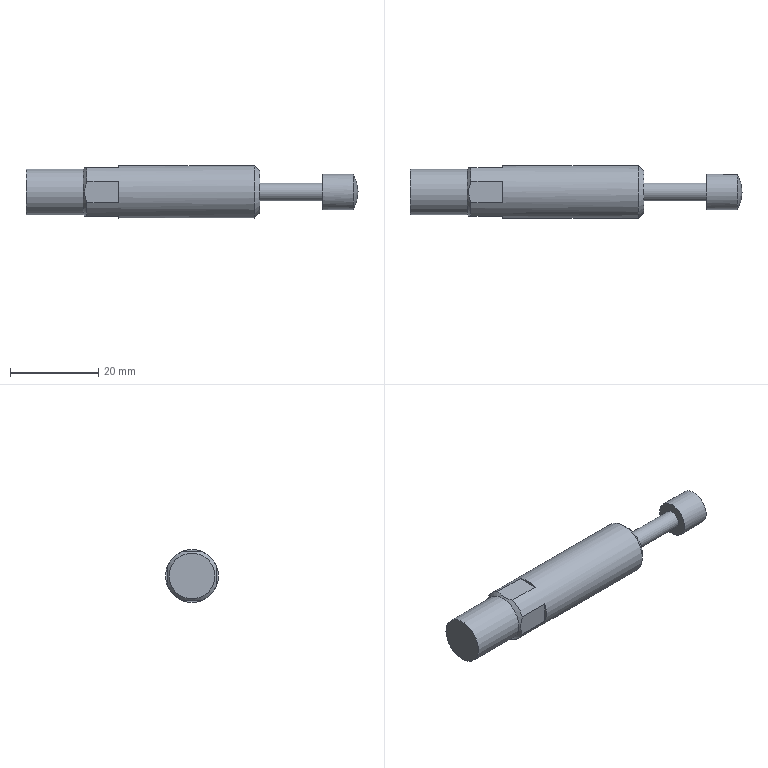Part | STEP file | 1 solid | 18 faces | box 75.3 x 12 x 12 mm | volume 6099 mm3 | plane 11 | cylinder 4 | cone 2 | sphere 1 | commonest cylinder face diameters 4 x1 8 x1 10.4 x1 12 x1